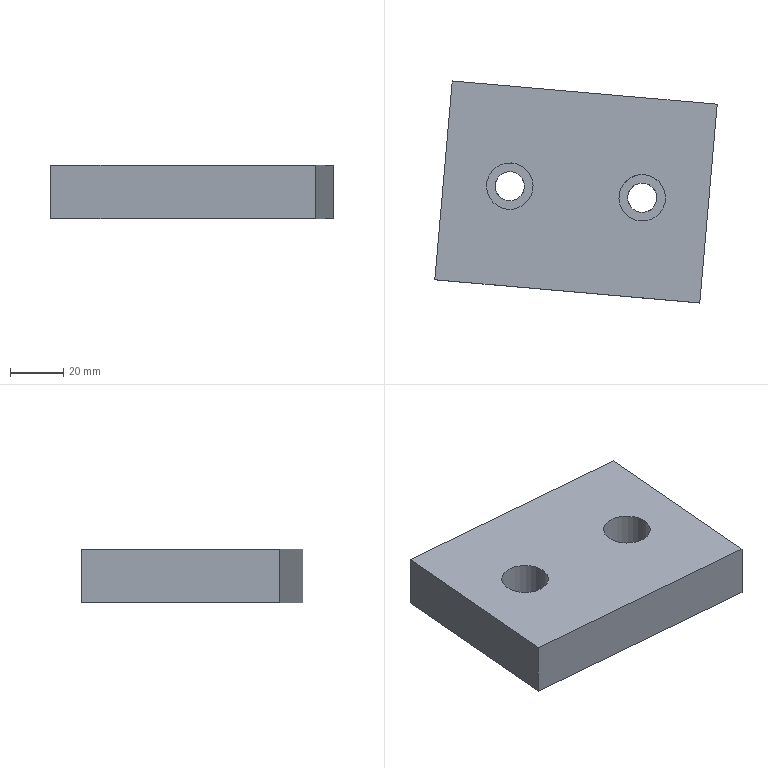Part | NX | features solid 2 | 1 solid | 12 faces | box 106.156 x 83.43 x 20 mm | volume 141834 mm3 | plane 8 | cylinder 4 | commonest cylinder face diameters 11 x2 17.5 x2
STEP:
#1=CARTESIAN_POINT('',(-645.805,650.009,-320.));
#2=VERTEX_POINT('',#1);
#3=CARTESIAN_POINT('',(-645.043,658.726,-320.));
#4=DIRECTION('',(0.,0.,-1.));
#5=DIRECTION('',(-0.08716,-0.9962,0.));
#6=AXIS2_PLACEMENT_3D('',#3,#4,#5);
#7=CIRCLE('',#6,8.75);
#8=EDGE_CURVE('',#2,#2,#7,.T.);
#9=ORIENTED_EDGE('',*,*,#8,.F.);
#10=EDGE_LOOP('',(#9));
#11=FACE_BOUND('',#10,.T.);
#12=CARTESIAN_POINT('',(-645.998,653.309,-320.));
#13=VERTEX_POINT('',#12);
#14=CARTESIAN_POINT('',(-645.043,658.726,-320.));
#15=DIRECTION('',(0.,0.,1.));
#16=DIRECTION('',(-0.1736,-0.9848,0.));
#17=AXIS2_PLACEMENT_3D('',#14,#15,#16);
#18=CIRCLE('',#17,5.5);
#19=EDGE_CURVE('',#13,#13,#18,.F.);
#20=ORIENTED_EDGE('',*,*,#19,.T.);
#21=EDGE_LOOP('',(#20));
#22=FACE_BOUND('',#21,.T.);
#23=CARTESIAN_POINT('',(-645.043,658.726,-320.));
#24=DIRECTION('',(0.,0.,-1.));
#25=DIRECTION('',(0.08716,0.9962,0.));
#26=AXIS2_PLACEMENT_3D('',#23,#24,#25);
#27=PLANE('',#26);
#28=ADVANCED_FACE('',(#11,#22),#27,.F.);
#29=CARTESIAN_POINT('',(-723.026,627.905,-305.));
#30=VERTEX_POINT('',#29);
#31=CARTESIAN_POINT('',(-716.489,702.62,-305.));
#32=VERTEX_POINT('',#31);
#33=CARTESIAN_POINT('',(-720.847,652.81,-305.));
#34=DIRECTION('',(0.08716,0.9962,0.));
#35=VECTOR('',#34,1000.);
#36=LINE('',#33,#35);
#37=EDGE_CURVE('',#30,#32,#36,.T.);
#38=ORIENTED_EDGE('',*,*,#37,.F.);
#39=CARTESIAN_POINT('',(-623.406,619.19,-305.));
#40=VERTEX_POINT('',#39);
#41=CARTESIAN_POINT('',(-673.216,623.547,-305.));
#42=DIRECTION('',(-0.9962,0.08716,0.));
#43=VECTOR('',#42,1000.);
#44=LINE('',#41,#43);
#45=EDGE_CURVE('',#40,#30,#44,.T.);
#46=ORIENTED_EDGE('',*,*,#45,.F.);
#47=CARTESIAN_POINT('',(-616.87,693.904,-305.));
#48=VERTEX_POINT('',#47);
#49=CARTESIAN_POINT('',(-621.227,644.095,-305.));
#50=DIRECTION('',(-0.08716,-0.9962,0.));
#51=VECTOR('',#50,1000.);
#52=LINE('',#49,#51);
#53=EDGE_CURVE('',#48,#40,#52,.T.);
#54=ORIENTED_EDGE('',*,*,#53,.F.);
#55=CARTESIAN_POINT('',(-666.679,698.262,-305.));
#56=DIRECTION('',(-0.9962,0.08716,0.));
#57=VECTOR('',#56,1000.);
#58=LINE('',#55,#57);
#59=EDGE_CURVE('',#48,#32,#58,.T.);
#60=ORIENTED_EDGE('',*,*,#59,.T.);
#61=EDGE_LOOP('',(#38,#46,#54,#60));
#62=FACE_BOUND('',#61,.T.);
#63=CARTESIAN_POINT('',(-644.28,667.443,-305.));
#64=VERTEX_POINT('',#63);
#65=CARTESIAN_POINT('',(-645.043,658.726,-305.));
#66=DIRECTION('',(0.,0.,1.));
#67=DIRECTION('',(0.08716,0.9962,0.));
#68=AXIS2_PLACEMENT_3D('',#65,#66,#67);
#69=CIRCLE('',#68,8.75);
#70=EDGE_CURVE('',#64,#64,#69,.T.);
#71=ORIENTED_EDGE('',*,*,#70,.F.);
#72=EDGE_LOOP('',(#71));
#73=FACE_BOUND('',#72,.T.);
#74=CARTESIAN_POINT('',(-694.09,671.8,-305.));
#75=VERTEX_POINT('',#74);
#76=CARTESIAN_POINT('',(-694.853,663.084,-305.));
#77=DIRECTION('',(0.,0.,1.));
#78=DIRECTION('',(0.08716,0.9962,0.));
#79=AXIS2_PLACEMENT_3D('',#76,#77,#78);
#80=CIRCLE('',#79,8.75);
#81=EDGE_CURVE('',#75,#75,#80,.T.);
#82=ORIENTED_EDGE('',*,*,#81,.F.);
#83=EDGE_LOOP('',(#82));
#84=FACE_BOUND('',#83,.T.);
#85=CARTESIAN_POINT('',(-671.037,648.452,-305.));
#86=DIRECTION('',(0.,0.,1.));
#87=DIRECTION('',(0.9962,-0.08716,0.));
#88=AXIS2_PLACEMENT_3D('',#85,#86,#87);
#89=PLANE('',#88);
#90=ADVANCED_FACE('',(#62,#73,#84),#89,.T.);
#91=ORIENTED_EDGE('',*,*,#70,.T.);
#92=EDGE_LOOP('',(#91));
#93=FACE_BOUND('',#92,.T.);
#94=ORIENTED_EDGE('',*,*,#8,.T.);
#95=EDGE_LOOP('',(#94));
#96=FACE_BOUND('',#95,.T.);
#97=CARTESIAN_POINT('',(-645.043,658.726,-320.));
#98=DIRECTION('',(0.,0.,1.));
#99=DIRECTION('',(-0.08716,-0.9962,0.));
#100=AXIS2_PLACEMENT_3D('',#97,#98,#99);
#101=CYLINDRICAL_SURFACE('',#100,8.75);
#102=ADVANCED_FACE('',(#93,#96),#101,.F.);
#103=ORIENTED_EDGE('',*,*,#19,.F.);
#104=EDGE_LOOP('',(#103));
#105=FACE_BOUND('',#104,.T.);
#106=CARTESIAN_POINT('',(-645.522,653.247,-325.));
#107=VERTEX_POINT('',#106);
#108=CARTESIAN_POINT('',(-645.043,658.726,-325.));
#109=DIRECTION('',(0.,0.,-1.));
#110=DIRECTION('',(-0.08716,-0.9962,0.));
#111=AXIS2_PLACEMENT_3D('',#108,#109,#110);
#112=CIRCLE('',#111,5.5);
#113=EDGE_CURVE('',#107,#107,#112,.T.);
#114=ORIENTED_EDGE('',*,*,#113,.T.);
#115=EDGE_LOOP('',(#114));
#116=FACE_BOUND('',#115,.T.);
#117=CARTESIAN_POINT('',(-645.043,658.726,-325.));
#118=DIRECTION('',(0.,0.,1.));
#119=DIRECTION('',(-0.08716,-0.9962,0.));
#120=AXIS2_PLACEMENT_3D('',#117,#118,#119);
#121=CYLINDRICAL_SURFACE('',#120,5.5);
#122=ADVANCED_FACE('',(#105,#116),#121,.F.);
#123=CARTESIAN_POINT('',(-623.406,619.19,-325.));
#124=VERTEX_POINT('',#123);
#125=CARTESIAN_POINT('',(-623.406,619.19,-315.));
#126=DIRECTION('',(0.,0.,-1.));
#127=VECTOR('',#126,1000.);
#128=LINE('',#125,#127);
#129=EDGE_CURVE('',#40,#124,#128,.T.);
#130=ORIENTED_EDGE('',*,*,#129,.T.);
#131=CARTESIAN_POINT('',(-616.87,693.904,-325.));
#132=VERTEX_POINT('',#131);
#133=CARTESIAN_POINT('',(-621.227,644.095,-325.));
#134=DIRECTION('',(0.08716,0.9962,0.));
#135=VECTOR('',#134,1000.);
#136=LINE('',#133,#135);
#137=EDGE_CURVE('',#124,#132,#136,.T.);
#138=ORIENTED_EDGE('',*,*,#137,.T.);
#139=CARTESIAN_POINT('',(-616.87,693.904,-315.));
#140=DIRECTION('',(0.,0.,1.));
#141=VECTOR('',#140,1000.);
#142=LINE('',#139,#141);
#143=EDGE_CURVE('',#132,#48,#142,.T.);
#144=ORIENTED_EDGE('',*,*,#143,.T.);
#145=ORIENTED_EDGE('',*,*,#53,.T.);
#146=EDGE_LOOP('',(#130,#138,#144,#145));
#147=FACE_BOUND('',#146,.T.);
#148=CARTESIAN_POINT('',(-621.227,644.095,-315.));
#149=DIRECTION('',(0.9962,-0.08716,0.));
#150=DIRECTION('',(0.,0.,-1.));
#151=AXIS2_PLACEMENT_3D('',#148,#149,#150);
#152=PLANE('',#151);
#153=ADVANCED_FACE('',(#147),#152,.T.);
#154=CARTESIAN_POINT('',(-723.026,627.905,-325.));
#155=VERTEX_POINT('',#154);
#156=CARTESIAN_POINT('',(-723.026,627.905,-315.));
#157=DIRECTION('',(0.,0.,1.));
#158=VECTOR('',#157,1000.);
#159=LINE('',#156,#158);
#160=EDGE_CURVE('',#155,#30,#159,.T.);
#161=ORIENTED_EDGE('',*,*,#160,.F.);
#162=CARTESIAN_POINT('',(-673.216,623.547,-325.));
#163=DIRECTION('',(-0.9962,0.08716,0.));
#164=VECTOR('',#163,1000.);
#165=LINE('',#162,#164);
#166=EDGE_CURVE('',#124,#155,#165,.T.);
#167=ORIENTED_EDGE('',*,*,#166,.F.);
#168=ORIENTED_EDGE('',*,*,#129,.F.);
#169=ORIENTED_EDGE('',*,*,#45,.T.);
#170=EDGE_LOOP('',(#161,#167,#168,#169));
#171=FACE_BOUND('',#170,.T.);
#172=CARTESIAN_POINT('',(-673.216,623.547,-315.));
#173=DIRECTION('',(-0.08716,-0.9962,0.));
#174=DIRECTION('',(-0.9962,0.08716,0.));
#175=AXIS2_PLACEMENT_3D('',#172,#173,#174);
#176=PLANE('',#175);
#177=ADVANCED_FACE('',(#171),#176,.T.);
#178=CARTESIAN_POINT('',(-716.489,702.62,-325.));
#179=VERTEX_POINT('',#178);
#180=CARTESIAN_POINT('',(-720.847,652.81,-325.));
#181=DIRECTION('',(0.08716,0.9962,0.));
#182=VECTOR('',#181,1000.);
#183=LINE('',#180,#182);
#184=EDGE_CURVE('',#179,#155,#183,.F.);
#185=ORIENTED_EDGE('',*,*,#184,.F.);
#186=CARTESIAN_POINT('',(-666.679,698.262,-325.));
#187=DIRECTION('',(-0.9962,0.08716,0.));
#188=VECTOR('',#187,1000.);
#189=LINE('',#186,#188);
#190=EDGE_CURVE('',#132,#179,#189,.T.);
#191=ORIENTED_EDGE('',*,*,#190,.F.);
#192=ORIENTED_EDGE('',*,*,#137,.F.);
#193=ORIENTED_EDGE('',*,*,#166,.T.);
#194=EDGE_LOOP('',(#185,#191,#192,#193));
#195=FACE_BOUND('',#194,.T.);
#196=ORIENTED_EDGE('',*,*,#113,.F.);
#197=EDGE_LOOP('',(#196));
#198=FACE_BOUND('',#197,.T.);
#199=CARTESIAN_POINT('',(-695.332,657.605,-325.));
#200=VERTEX_POINT('',#199);
#201=CARTESIAN_POINT('',(-694.853,663.084,-325.));
#202=DIRECTION('',(0.,0.,-1.));
#203=DIRECTION('',(-0.08716,-0.9962,0.));
#204=AXIS2_PLACEMENT_3D('',#201,#202,#203);
#205=CIRCLE('',#204,5.5);
#206=EDGE_CURVE('',#200,#200,#205,.T.);
#207=ORIENTED_EDGE('',*,*,#206,.F.);
#208=EDGE_LOOP('',(#207));
#209=FACE_BOUND('',#208,.T.);
#210=CARTESIAN_POINT('',(-671.037,648.452,-325.));
#211=DIRECTION('',(0.,0.,-1.));
#212=DIRECTION('',(-0.9962,0.08716,0.));
#213=AXIS2_PLACEMENT_3D('',#210,#211,#212);
#214=PLANE('',#213);
#215=ADVANCED_FACE('',(#195,#198,#209),#214,.T.);
#216=ORIENTED_EDGE('',*,*,#190,.T.);
#217=CARTESIAN_POINT('',(-716.489,702.62,-315.));
#218=DIRECTION('',(0.,0.,-1.));
#219=VECTOR('',#218,1000.);
#220=LINE('',#217,#219);
#221=EDGE_CURVE('',#32,#179,#220,.T.);
#222=ORIENTED_EDGE('',*,*,#221,.F.);
#223=ORIENTED_EDGE('',*,*,#59,.F.);
#224=ORIENTED_EDGE('',*,*,#143,.F.);
#225=EDGE_LOOP('',(#216,#222,#223,#224));
#226=FACE_BOUND('',#225,.T.);
#227=CARTESIAN_POINT('',(-666.679,698.262,-315.));
#228=DIRECTION('',(0.08716,0.9962,0.));
#229=DIRECTION('',(0.9962,-0.08716,0.));
#230=AXIS2_PLACEMENT_3D('',#227,#228,#229);
#231=PLANE('',#230);
#232=ADVANCED_FACE('',(#226),#231,.T.);
#233=CARTESIAN_POINT('',(-695.615,654.367,-320.));
#234=VERTEX_POINT('',#233);
#235=CARTESIAN_POINT('',(-694.853,663.084,-320.));
#236=DIRECTION('',(0.,0.,-1.));
#237=DIRECTION('',(-0.08716,-0.9962,0.));
#238=AXIS2_PLACEMENT_3D('',#235,#236,#237);
#239=CIRCLE('',#238,8.75);
#240=EDGE_CURVE('',#234,#234,#239,.T.);
#241=ORIENTED_EDGE('',*,*,#240,.F.);
#242=EDGE_LOOP('',(#241));
#243=FACE_BOUND('',#242,.T.);
#244=CARTESIAN_POINT('',(-695.808,657.667,-320.));
#245=VERTEX_POINT('',#244);
#246=CARTESIAN_POINT('',(-694.853,663.084,-320.));
#247=DIRECTION('',(0.,0.,1.));
#248=DIRECTION('',(-0.1736,-0.9848,0.));
#249=AXIS2_PLACEMENT_3D('',#246,#247,#248);
#250=CIRCLE('',#249,5.5);
#251=EDGE_CURVE('',#245,#245,#250,.F.);
#252=ORIENTED_EDGE('',*,*,#251,.T.);
#253=EDGE_LOOP('',(#252));
#254=FACE_BOUND('',#253,.T.);
#255=CARTESIAN_POINT('',(-694.853,663.084,-320.));
#256=DIRECTION('',(0.,0.,-1.));
#257=DIRECTION('',(0.08716,0.9962,0.));
#258=AXIS2_PLACEMENT_3D('',#255,#256,#257);
#259=PLANE('',#258);
#260=ADVANCED_FACE('',(#243,#254),#259,.F.);
#261=ORIENTED_EDGE('',*,*,#251,.F.);
#262=EDGE_LOOP('',(#261));
#263=FACE_BOUND('',#262,.T.);
#264=ORIENTED_EDGE('',*,*,#206,.T.);
#265=EDGE_LOOP('',(#264));
#266=FACE_BOUND('',#265,.T.);
#267=CARTESIAN_POINT('',(-694.853,663.084,-325.));
#268=DIRECTION('',(0.,0.,1.));
#269=DIRECTION('',(-0.08716,-0.9962,0.));
#270=AXIS2_PLACEMENT_3D('',#267,#268,#269);
#271=CYLINDRICAL_SURFACE('',#270,5.5);
#272=ADVANCED_FACE('',(#263,#266),#271,.F.);
#273=ORIENTED_EDGE('',*,*,#81,.T.);
#274=EDGE_LOOP('',(#273));
#275=FACE_BOUND('',#274,.T.);
#276=ORIENTED_EDGE('',*,*,#240,.T.);
#277=EDGE_LOOP('',(#276));
#278=FACE_BOUND('',#277,.T.);
#279=CARTESIAN_POINT('',(-694.853,663.084,-320.));
#280=DIRECTION('',(0.,0.,1.));
#281=DIRECTION('',(-0.08716,-0.9962,0.));
#282=AXIS2_PLACEMENT_3D('',#279,#280,#281);
#283=CYLINDRICAL_SURFACE('',#282,8.75);
#284=ADVANCED_FACE('',(#275,#278),#283,.F.);
#285=ORIENTED_EDGE('',*,*,#221,.T.);
#286=ORIENTED_EDGE('',*,*,#184,.T.);
#287=ORIENTED_EDGE('',*,*,#160,.T.);
#288=ORIENTED_EDGE('',*,*,#37,.T.);
#289=EDGE_LOOP('',(#285,#286,#287,#288));
#290=FACE_BOUND('',#289,.T.);
#291=CARTESIAN_POINT('',(-720.847,652.81,-315.));
#292=DIRECTION('',(-0.9962,0.08716,0.));
#293=DIRECTION('',(0.,0.,1.));
#294=AXIS2_PLACEMENT_3D('',#291,#292,#293);
#295=PLANE('',#294);
#296=ADVANCED_FACE('',(#290),#295,.T.);
#297=CLOSED_SHELL('',(#28,#90,#102,#122,#153,#177,#215,#232,#260,#272,#284,#296));
#298=MANIFOLD_SOLID_BREP('',#297);
#299=(LENGTH_UNIT()NAMED_UNIT(*)SI_UNIT(.MILLI.,.METRE.));
#300=UNCERTAINTY_MEASURE_WITH_UNIT(LENGTH_MEASURE(0.00001),#299,'','');
#301=(NAMED_UNIT(*)PLANE_ANGLE_UNIT()SI_UNIT($,.RADIAN.));
#302=(NAMED_UNIT(*)SI_UNIT($,.STERADIAN.)SOLID_ANGLE_UNIT());
#303=(GEOMETRIC_REPRESENTATION_CONTEXT(3)GLOBAL_UNCERTAINTY_ASSIGNED_CONTEXT((#300))GLOBAL_UNIT_ASSIGNED_CONTEXT((#299,#301,#302))REPRESENTATION_CONTEXT('',''));
#304=ADVANCED_BREP_SHAPE_REPRESENTATION('',(#298),#303);